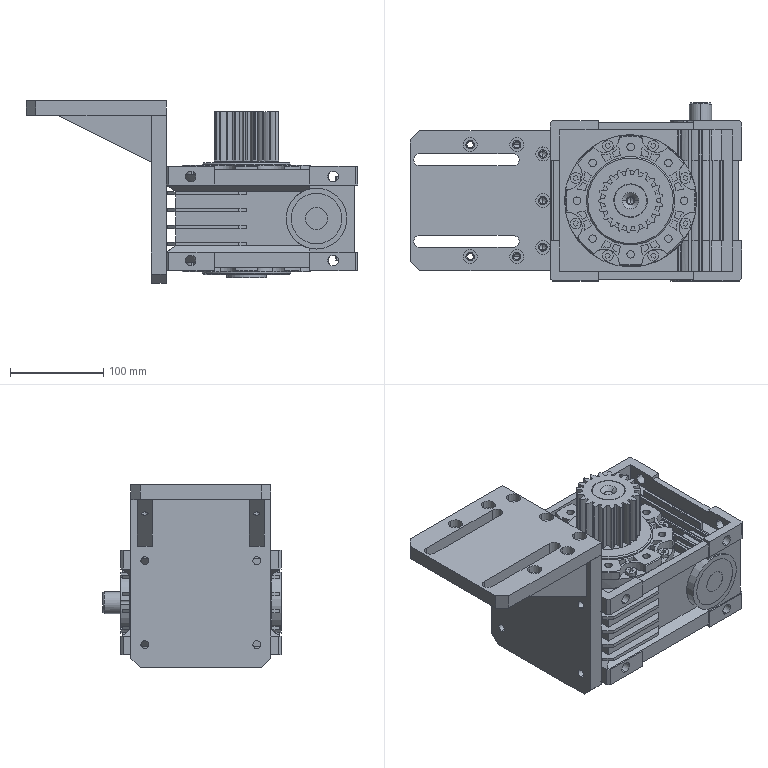Part | SolidWorks | 10 solids | 1152 faces | box 355 x 191 x 196 mm | volume 4077245 mm3 | cylinder 543 | plane 535 | cone 74 | commonest cylinder face diameters 1 x80 11.5 x64 25.2 x46 36.765 x36 8 x34 99.75 x32